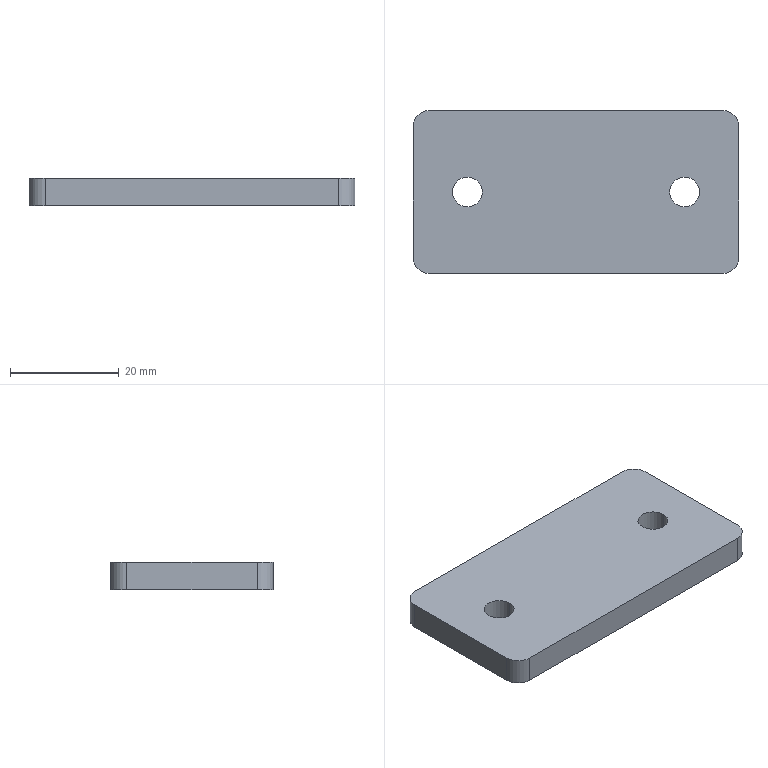Part | STEP file | Guide wheel mechanism revised.sldasm-Part-42 | 1 solid | 14 faces | box 60 x 30 x 5 mm | volume 8724 mm3 | cylinder 8 | plane 6 | commonest cylinder face diameters 5.5 x4 6 x4
STEP:
#1=CARTESIAN_POINT('',(-17.25,0.,-2.5));
#2=VERTEX_POINT('',#1);
#3=CARTESIAN_POINT('',(-22.75,0.,-2.5));
#4=VERTEX_POINT('',#3);
#5=CARTESIAN_POINT('',(-20.,0.,-2.5));
#6=DIRECTION('',(0.,0.,-1.));
#7=DIRECTION('',(-1.,0.,0.));
#8=AXIS2_PLACEMENT_3D('',#5,#6,#7);
#9=CIRCLE('',#8,2.75);
#10=EDGE_CURVE('',#2,#4,#9,.T.);
#11=ORIENTED_EDGE('',*,*,#10,.T.);
#12=CARTESIAN_POINT('',(-22.75,0.,2.5));
#13=VERTEX_POINT('',#12);
#14=CARTESIAN_POINT('',(-22.75,0.,2.5));
#15=DIRECTION('',(0.,0.,1.));
#16=VECTOR('',#15,1000.);
#17=LINE('',#14,#16);
#18=EDGE_CURVE('',#4,#13,#17,.T.);
#19=ORIENTED_EDGE('',*,*,#18,.T.);
#20=CARTESIAN_POINT('',(-17.25,0.,2.5));
#21=VERTEX_POINT('',#20);
#22=CARTESIAN_POINT('',(-20.,0.,2.5));
#23=DIRECTION('',(0.,0.,1.));
#24=DIRECTION('',(1.,0.,0.));
#25=AXIS2_PLACEMENT_3D('',#22,#23,#24);
#26=CIRCLE('',#25,2.75);
#27=EDGE_CURVE('',#13,#21,#26,.T.);
#28=ORIENTED_EDGE('',*,*,#27,.T.);
#29=CARTESIAN_POINT('',(-17.25,0.,2.5));
#30=DIRECTION('',(0.,0.,1.));
#31=VECTOR('',#30,1000.);
#32=LINE('',#29,#31);
#33=EDGE_CURVE('',#2,#21,#32,.T.);
#34=ORIENTED_EDGE('',*,*,#33,.F.);
#35=EDGE_LOOP('',(#11,#19,#28,#34));
#36=FACE_OUTER_BOUND('',#35,.T.);
#37=CARTESIAN_POINT('',(-20.,0.,2.5));
#38=DIRECTION('',(0.,0.,1.));
#39=DIRECTION('',(1.,0.,0.));
#40=AXIS2_PLACEMENT_3D('',#37,#38,#39);
#41=CYLINDRICAL_SURFACE('',#40,2.75);
#42=ADVANCED_FACE('',(#36),#41,.F.);
#43=CARTESIAN_POINT('',(22.75,0.,-2.5));
#44=VERTEX_POINT('',#43);
#45=CARTESIAN_POINT('',(17.25,0.,-2.5));
#46=VERTEX_POINT('',#45);
#47=CARTESIAN_POINT('',(20.,0.,-2.5));
#48=DIRECTION('',(0.,0.,-1.));
#49=DIRECTION('',(-1.,0.,0.));
#50=AXIS2_PLACEMENT_3D('',#47,#48,#49);
#51=CIRCLE('',#50,2.75);
#52=EDGE_CURVE('',#44,#46,#51,.T.);
#53=ORIENTED_EDGE('',*,*,#52,.T.);
#54=CARTESIAN_POINT('',(17.25,0.,2.5));
#55=VERTEX_POINT('',#54);
#56=CARTESIAN_POINT('',(17.25,0.,2.5));
#57=DIRECTION('',(0.,0.,1.));
#58=VECTOR('',#57,1000.);
#59=LINE('',#56,#58);
#60=EDGE_CURVE('',#46,#55,#59,.T.);
#61=ORIENTED_EDGE('',*,*,#60,.T.);
#62=CARTESIAN_POINT('',(22.75,0.,2.5));
#63=VERTEX_POINT('',#62);
#64=CARTESIAN_POINT('',(20.,0.,2.5));
#65=DIRECTION('',(0.,0.,1.));
#66=DIRECTION('',(1.,0.,0.));
#67=AXIS2_PLACEMENT_3D('',#64,#65,#66);
#68=CIRCLE('',#67,2.75);
#69=EDGE_CURVE('',#55,#63,#68,.T.);
#70=ORIENTED_EDGE('',*,*,#69,.T.);
#71=CARTESIAN_POINT('',(22.75,0.,2.5));
#72=DIRECTION('',(0.,0.,1.));
#73=VECTOR('',#72,1000.);
#74=LINE('',#71,#73);
#75=EDGE_CURVE('',#44,#63,#74,.T.);
#76=ORIENTED_EDGE('',*,*,#75,.F.);
#77=EDGE_LOOP('',(#53,#61,#70,#76));
#78=FACE_OUTER_BOUND('',#77,.T.);
#79=CARTESIAN_POINT('',(20.,0.,2.5));
#80=DIRECTION('',(0.,0.,1.));
#81=DIRECTION('',(1.,0.,0.));
#82=AXIS2_PLACEMENT_3D('',#79,#80,#81);
#83=CYLINDRICAL_SURFACE('',#82,2.75);
#84=ADVANCED_FACE('',(#78),#83,.F.);
#85=CARTESIAN_POINT('',(30.,-12.,2.5));
#86=VERTEX_POINT('',#85);
#87=CARTESIAN_POINT('',(30.,12.,2.5));
#88=VERTEX_POINT('',#87);
#89=CARTESIAN_POINT('',(30.,-15.,2.5));
#90=DIRECTION('',(0.,1.,0.));
#91=VECTOR('',#90,1000.);
#92=LINE('',#89,#91);
#93=EDGE_CURVE('',#86,#88,#92,.T.);
#94=ORIENTED_EDGE('',*,*,#93,.F.);
#95=CARTESIAN_POINT('',(30.,-12.,-2.5));
#96=VERTEX_POINT('',#95);
#97=CARTESIAN_POINT('',(30.,-12.,2.5));
#98=DIRECTION('',(0.,0.,-1.));
#99=VECTOR('',#98,1000.);
#100=LINE('',#97,#99);
#101=EDGE_CURVE('',#86,#96,#100,.T.);
#102=ORIENTED_EDGE('',*,*,#101,.T.);
#103=CARTESIAN_POINT('',(30.,12.,-2.5));
#104=VERTEX_POINT('',#103);
#105=CARTESIAN_POINT('',(30.,-15.,-2.5));
#106=DIRECTION('',(0.,1.,0.));
#107=VECTOR('',#106,1000.);
#108=LINE('',#105,#107);
#109=EDGE_CURVE('',#96,#104,#108,.T.);
#110=ORIENTED_EDGE('',*,*,#109,.T.);
#111=CARTESIAN_POINT('',(30.,12.,2.5));
#112=DIRECTION('',(0.,0.,1.));
#113=VECTOR('',#112,1000.);
#114=LINE('',#111,#113);
#115=EDGE_CURVE('',#104,#88,#114,.T.);
#116=ORIENTED_EDGE('',*,*,#115,.T.);
#117=EDGE_LOOP('',(#94,#102,#110,#116));
#118=FACE_OUTER_BOUND('',#117,.T.);
#119=CARTESIAN_POINT('',(30.,-15.,2.5));
#120=DIRECTION('',(-1.,0.,0.));
#121=DIRECTION('',(0.,0.,1.));
#122=AXIS2_PLACEMENT_3D('',#119,#120,#121);
#123=PLANE('',#122);
#124=ADVANCED_FACE('',(#118),#123,.F.);
#125=CARTESIAN_POINT('',(27.,15.,-2.5));
#126=VERTEX_POINT('',#125);
#127=CARTESIAN_POINT('',(-27.,15.,-2.5));
#128=VERTEX_POINT('',#127);
#129=CARTESIAN_POINT('',(-30.,15.,-2.5));
#130=DIRECTION('',(-1.,0.,0.));
#131=VECTOR('',#130,1000.);
#132=LINE('',#129,#131);
#133=EDGE_CURVE('',#126,#128,#132,.T.);
#134=ORIENTED_EDGE('',*,*,#133,.T.);
#135=CARTESIAN_POINT('',(-27.,15.,2.5));
#136=VERTEX_POINT('',#135);
#137=CARTESIAN_POINT('',(-27.,15.,2.5));
#138=DIRECTION('',(0.,0.,1.));
#139=VECTOR('',#138,1000.);
#140=LINE('',#137,#139);
#141=EDGE_CURVE('',#128,#136,#140,.T.);
#142=ORIENTED_EDGE('',*,*,#141,.T.);
#143=CARTESIAN_POINT('',(27.,15.,2.5));
#144=VERTEX_POINT('',#143);
#145=CARTESIAN_POINT('',(-30.,15.,2.5));
#146=DIRECTION('',(-1.,0.,0.));
#147=VECTOR('',#146,1000.);
#148=LINE('',#145,#147);
#149=EDGE_CURVE('',#144,#136,#148,.T.);
#150=ORIENTED_EDGE('',*,*,#149,.F.);
#151=CARTESIAN_POINT('',(27.,15.,2.5));
#152=DIRECTION('',(0.,0.,-1.));
#153=VECTOR('',#152,1000.);
#154=LINE('',#151,#153);
#155=EDGE_CURVE('',#144,#126,#154,.T.);
#156=ORIENTED_EDGE('',*,*,#155,.T.);
#157=EDGE_LOOP('',(#134,#142,#150,#156));
#158=FACE_OUTER_BOUND('',#157,.T.);
#159=CARTESIAN_POINT('',(-30.,15.,2.5));
#160=DIRECTION('',(0.,-1.,0.));
#161=DIRECTION('',(0.,0.,-1.));
#162=AXIS2_PLACEMENT_3D('',#159,#160,#161);
#163=PLANE('',#162);
#164=ADVANCED_FACE('',(#158),#163,.F.);
#165=CARTESIAN_POINT('',(-30.,12.,-2.5));
#166=VERTEX_POINT('',#165);
#167=CARTESIAN_POINT('',(-30.,-12.,-2.5));
#168=VERTEX_POINT('',#167);
#169=CARTESIAN_POINT('',(-30.,-15.,-2.5));
#170=DIRECTION('',(0.,-1.,0.));
#171=VECTOR('',#170,1000.);
#172=LINE('',#169,#171);
#173=EDGE_CURVE('',#166,#168,#172,.T.);
#174=ORIENTED_EDGE('',*,*,#173,.T.);
#175=CARTESIAN_POINT('',(-30.,-12.,2.5));
#176=VERTEX_POINT('',#175);
#177=CARTESIAN_POINT('',(-30.,-12.,2.5));
#178=DIRECTION('',(0.,0.,1.));
#179=VECTOR('',#178,1000.);
#180=LINE('',#177,#179);
#181=EDGE_CURVE('',#168,#176,#180,.T.);
#182=ORIENTED_EDGE('',*,*,#181,.T.);
#183=CARTESIAN_POINT('',(-30.,12.,2.5));
#184=VERTEX_POINT('',#183);
#185=CARTESIAN_POINT('',(-30.,-15.,2.5));
#186=DIRECTION('',(0.,-1.,0.));
#187=VECTOR('',#186,1000.);
#188=LINE('',#185,#187);
#189=EDGE_CURVE('',#184,#176,#188,.T.);
#190=ORIENTED_EDGE('',*,*,#189,.F.);
#191=CARTESIAN_POINT('',(-30.,12.,2.5));
#192=DIRECTION('',(0.,0.,-1.));
#193=VECTOR('',#192,1000.);
#194=LINE('',#191,#193);
#195=EDGE_CURVE('',#184,#166,#194,.T.);
#196=ORIENTED_EDGE('',*,*,#195,.T.);
#197=EDGE_LOOP('',(#174,#182,#190,#196));
#198=FACE_OUTER_BOUND('',#197,.T.);
#199=CARTESIAN_POINT('',(-30.,-15.,2.5));
#200=DIRECTION('',(1.,0.,0.));
#201=DIRECTION('',(0.,0.,-1.));
#202=AXIS2_PLACEMENT_3D('',#199,#200,#201);
#203=PLANE('',#202);
#204=ADVANCED_FACE('',(#198),#203,.F.);
#205=CARTESIAN_POINT('',(-27.,-15.,2.5));
#206=VERTEX_POINT('',#205);
#207=CARTESIAN_POINT('',(27.,-15.,2.5));
#208=VERTEX_POINT('',#207);
#209=CARTESIAN_POINT('',(-30.,-15.,2.5));
#210=DIRECTION('',(1.,0.,0.));
#211=VECTOR('',#210,1000.);
#212=LINE('',#209,#211);
#213=EDGE_CURVE('',#206,#208,#212,.T.);
#214=ORIENTED_EDGE('',*,*,#213,.F.);
#215=CARTESIAN_POINT('',(-27.,-15.,-2.5));
#216=VERTEX_POINT('',#215);
#217=CARTESIAN_POINT('',(-27.,-15.,2.5));
#218=DIRECTION('',(0.,0.,-1.));
#219=VECTOR('',#218,1000.);
#220=LINE('',#217,#219);
#221=EDGE_CURVE('',#206,#216,#220,.T.);
#222=ORIENTED_EDGE('',*,*,#221,.T.);
#223=CARTESIAN_POINT('',(27.,-15.,-2.5));
#224=VERTEX_POINT('',#223);
#225=CARTESIAN_POINT('',(-30.,-15.,-2.5));
#226=DIRECTION('',(1.,0.,0.));
#227=VECTOR('',#226,1000.);
#228=LINE('',#225,#227);
#229=EDGE_CURVE('',#216,#224,#228,.T.);
#230=ORIENTED_EDGE('',*,*,#229,.T.);
#231=CARTESIAN_POINT('',(27.,-15.,2.5));
#232=DIRECTION('',(0.,0.,1.));
#233=VECTOR('',#232,1000.);
#234=LINE('',#231,#233);
#235=EDGE_CURVE('',#224,#208,#234,.T.);
#236=ORIENTED_EDGE('',*,*,#235,.T.);
#237=EDGE_LOOP('',(#214,#222,#230,#236));
#238=FACE_OUTER_BOUND('',#237,.T.);
#239=CARTESIAN_POINT('',(-30.,-15.,2.5));
#240=DIRECTION('',(0.,1.,0.));
#241=DIRECTION('',(0.,0.,1.));
#242=AXIS2_PLACEMENT_3D('',#239,#240,#241);
#243=PLANE('',#242);
#244=ADVANCED_FACE('',(#238),#243,.F.);
#245=CARTESIAN_POINT('',(-20.,0.,2.5));
#246=DIRECTION('',(0.,0.,1.));
#247=DIRECTION('',(1.,0.,0.));
#248=AXIS2_PLACEMENT_3D('',#245,#246,#247);
#249=CIRCLE('',#248,2.75);
#250=EDGE_CURVE('',#21,#13,#249,.T.);
#251=ORIENTED_EDGE('',*,*,#250,.F.);
#252=ORIENTED_EDGE('',*,*,#27,.F.);
#253=EDGE_LOOP('',(#251,#252));
#254=FACE_BOUND('',#253,.T.);
#255=CARTESIAN_POINT('',(20.,0.,2.5));
#256=DIRECTION('',(0.,0.,1.));
#257=DIRECTION('',(1.,0.,0.));
#258=AXIS2_PLACEMENT_3D('',#255,#256,#257);
#259=CIRCLE('',#258,2.75);
#260=EDGE_CURVE('',#63,#55,#259,.T.);
#261=ORIENTED_EDGE('',*,*,#260,.F.);
#262=ORIENTED_EDGE('',*,*,#69,.F.);
#263=EDGE_LOOP('',(#261,#262));
#264=FACE_BOUND('',#263,.T.);
#265=ORIENTED_EDGE('',*,*,#189,.T.);
#266=CARTESIAN_POINT('',(-27.,-12.,2.5));
#267=DIRECTION('',(0.,0.,1.));
#268=DIRECTION('',(-1.,0.,0.));
#269=AXIS2_PLACEMENT_3D('',#266,#267,#268);
#270=CIRCLE('',#269,3.);
#271=EDGE_CURVE('',#176,#206,#270,.T.);
#272=ORIENTED_EDGE('',*,*,#271,.T.);
#273=ORIENTED_EDGE('',*,*,#213,.T.);
#274=CARTESIAN_POINT('',(27.,-12.,2.5));
#275=DIRECTION('',(0.,0.,1.));
#276=DIRECTION('',(-1.,0.,0.));
#277=AXIS2_PLACEMENT_3D('',#274,#275,#276);
#278=CIRCLE('',#277,3.);
#279=EDGE_CURVE('',#208,#86,#278,.T.);
#280=ORIENTED_EDGE('',*,*,#279,.T.);
#281=ORIENTED_EDGE('',*,*,#93,.T.);
#282=CARTESIAN_POINT('',(27.,12.,2.5));
#283=DIRECTION('',(0.,0.,1.));
#284=DIRECTION('',(-1.,0.,0.));
#285=AXIS2_PLACEMENT_3D('',#282,#283,#284);
#286=CIRCLE('',#285,3.);
#287=EDGE_CURVE('',#88,#144,#286,.T.);
#288=ORIENTED_EDGE('',*,*,#287,.T.);
#289=ORIENTED_EDGE('',*,*,#149,.T.);
#290=CARTESIAN_POINT('',(-27.,12.,2.5));
#291=DIRECTION('',(0.,0.,1.));
#292=DIRECTION('',(-1.,0.,0.));
#293=AXIS2_PLACEMENT_3D('',#290,#291,#292);
#294=CIRCLE('',#293,3.);
#295=EDGE_CURVE('',#136,#184,#294,.T.);
#296=ORIENTED_EDGE('',*,*,#295,.T.);
#297=EDGE_LOOP('',(#265,#272,#273,#280,#281,#288,#289,#296));
#298=FACE_OUTER_BOUND('',#297,.T.);
#299=CARTESIAN_POINT('',(0.,0.,2.5));
#300=DIRECTION('',(0.,0.,-1.));
#301=DIRECTION('',(-1.,0.,0.));
#302=AXIS2_PLACEMENT_3D('',#299,#300,#301);
#303=PLANE('',#302);
#304=ADVANCED_FACE('',(#254,#264,#298),#303,.F.);
#305=ORIENTED_EDGE('',*,*,#10,.F.);
#306=CARTESIAN_POINT('',(-20.,0.,-2.5));
#307=DIRECTION('',(0.,0.,-1.));
#308=DIRECTION('',(-1.,0.,0.));
#309=AXIS2_PLACEMENT_3D('',#306,#307,#308);
#310=CIRCLE('',#309,2.75);
#311=EDGE_CURVE('',#4,#2,#310,.T.);
#312=ORIENTED_EDGE('',*,*,#311,.F.);
#313=EDGE_LOOP('',(#305,#312));
#314=FACE_BOUND('',#313,.T.);
#315=ORIENTED_EDGE('',*,*,#52,.F.);
#316=CARTESIAN_POINT('',(20.,0.,-2.5));
#317=DIRECTION('',(0.,0.,-1.));
#318=DIRECTION('',(-1.,0.,0.));
#319=AXIS2_PLACEMENT_3D('',#316,#317,#318);
#320=CIRCLE('',#319,2.75);
#321=EDGE_CURVE('',#46,#44,#320,.T.);
#322=ORIENTED_EDGE('',*,*,#321,.F.);
#323=EDGE_LOOP('',(#315,#322));
#324=FACE_BOUND('',#323,.T.);
#325=ORIENTED_EDGE('',*,*,#229,.F.);
#326=CARTESIAN_POINT('',(-27.,-12.,-2.5));
#327=DIRECTION('',(0.,0.,-1.));
#328=DIRECTION('',(-1.,0.,0.));
#329=AXIS2_PLACEMENT_3D('',#326,#327,#328);
#330=CIRCLE('',#329,3.);
#331=EDGE_CURVE('',#216,#168,#330,.T.);
#332=ORIENTED_EDGE('',*,*,#331,.T.);
#333=ORIENTED_EDGE('',*,*,#173,.F.);
#334=CARTESIAN_POINT('',(-27.,12.,-2.5));
#335=DIRECTION('',(0.,0.,-1.));
#336=DIRECTION('',(-1.,0.,0.));
#337=AXIS2_PLACEMENT_3D('',#334,#335,#336);
#338=CIRCLE('',#337,3.);
#339=EDGE_CURVE('',#166,#128,#338,.T.);
#340=ORIENTED_EDGE('',*,*,#339,.T.);
#341=ORIENTED_EDGE('',*,*,#133,.F.);
#342=CARTESIAN_POINT('',(27.,12.,-2.5));
#343=DIRECTION('',(0.,0.,-1.));
#344=DIRECTION('',(-1.,0.,0.));
#345=AXIS2_PLACEMENT_3D('',#342,#343,#344);
#346=CIRCLE('',#345,3.);
#347=EDGE_CURVE('',#126,#104,#346,.T.);
#348=ORIENTED_EDGE('',*,*,#347,.T.);
#349=ORIENTED_EDGE('',*,*,#109,.F.);
#350=CARTESIAN_POINT('',(27.,-12.,-2.5));
#351=DIRECTION('',(0.,0.,-1.));
#352=DIRECTION('',(-1.,0.,0.));
#353=AXIS2_PLACEMENT_3D('',#350,#351,#352);
#354=CIRCLE('',#353,3.);
#355=EDGE_CURVE('',#96,#224,#354,.T.);
#356=ORIENTED_EDGE('',*,*,#355,.T.);
#357=EDGE_LOOP('',(#325,#332,#333,#340,#341,#348,#349,#356));
#358=FACE_OUTER_BOUND('',#357,.T.);
#359=CARTESIAN_POINT('',(0.,0.,-2.5));
#360=DIRECTION('',(0.,0.,-1.));
#361=DIRECTION('',(-1.,0.,0.));
#362=AXIS2_PLACEMENT_3D('',#359,#360,#361);
#363=PLANE('',#362);
#364=ADVANCED_FACE('',(#314,#324,#358),#363,.T.);
#365=ORIENTED_EDGE('',*,*,#60,.F.);
#366=ORIENTED_EDGE('',*,*,#321,.T.);
#367=ORIENTED_EDGE('',*,*,#75,.T.);
#368=ORIENTED_EDGE('',*,*,#260,.T.);
#369=EDGE_LOOP('',(#365,#366,#367,#368));
#370=FACE_OUTER_BOUND('',#369,.T.);
#371=CARTESIAN_POINT('',(20.,0.,2.5));
#372=DIRECTION('',(0.,0.,1.));
#373=DIRECTION('',(1.,0.,0.));
#374=AXIS2_PLACEMENT_3D('',#371,#372,#373);
#375=CYLINDRICAL_SURFACE('',#374,2.75);
#376=ADVANCED_FACE('',(#370),#375,.F.);
#377=ORIENTED_EDGE('',*,*,#18,.F.);
#378=ORIENTED_EDGE('',*,*,#311,.T.);
#379=ORIENTED_EDGE('',*,*,#33,.T.);
#380=ORIENTED_EDGE('',*,*,#250,.T.);
#381=EDGE_LOOP('',(#377,#378,#379,#380));
#382=FACE_OUTER_BOUND('',#381,.T.);
#383=CARTESIAN_POINT('',(-20.,0.,2.5));
#384=DIRECTION('',(0.,0.,1.));
#385=DIRECTION('',(1.,0.,0.));
#386=AXIS2_PLACEMENT_3D('',#383,#384,#385);
#387=CYLINDRICAL_SURFACE('',#386,2.75);
#388=ADVANCED_FACE('',(#382),#387,.F.);
#389=ORIENTED_EDGE('',*,*,#271,.F.);
#390=ORIENTED_EDGE('',*,*,#181,.F.);
#391=ORIENTED_EDGE('',*,*,#331,.F.);
#392=ORIENTED_EDGE('',*,*,#221,.F.);
#393=EDGE_LOOP('',(#389,#390,#391,#392));
#394=FACE_OUTER_BOUND('',#393,.T.);
#395=CARTESIAN_POINT('',(-27.,-12.,2.5));
#396=DIRECTION('',(0.,0.,-1.));
#397=DIRECTION('',(-1.,0.,0.));
#398=AXIS2_PLACEMENT_3D('',#395,#396,#397);
#399=CYLINDRICAL_SURFACE('',#398,3.);
#400=ADVANCED_FACE('',(#394),#399,.T.);
#401=ORIENTED_EDGE('',*,*,#279,.F.);
#402=ORIENTED_EDGE('',*,*,#235,.F.);
#403=ORIENTED_EDGE('',*,*,#355,.F.);
#404=ORIENTED_EDGE('',*,*,#101,.F.);
#405=EDGE_LOOP('',(#401,#402,#403,#404));
#406=FACE_OUTER_BOUND('',#405,.T.);
#407=CARTESIAN_POINT('',(27.,-12.,2.5));
#408=DIRECTION('',(0.,0.,-1.));
#409=DIRECTION('',(-1.,0.,0.));
#410=AXIS2_PLACEMENT_3D('',#407,#408,#409);
#411=CYLINDRICAL_SURFACE('',#410,3.);
#412=ADVANCED_FACE('',(#406),#411,.T.);
#413=ORIENTED_EDGE('',*,*,#295,.F.);
#414=ORIENTED_EDGE('',*,*,#141,.F.);
#415=ORIENTED_EDGE('',*,*,#339,.F.);
#416=ORIENTED_EDGE('',*,*,#195,.F.);
#417=EDGE_LOOP('',(#413,#414,#415,#416));
#418=FACE_OUTER_BOUND('',#417,.T.);
#419=CARTESIAN_POINT('',(-27.,12.,2.5));
#420=DIRECTION('',(0.,0.,-1.));
#421=DIRECTION('',(-1.,0.,0.));
#422=AXIS2_PLACEMENT_3D('',#419,#420,#421);
#423=CYLINDRICAL_SURFACE('',#422,3.);
#424=ADVANCED_FACE('',(#418),#423,.T.);
#425=ORIENTED_EDGE('',*,*,#287,.F.);
#426=ORIENTED_EDGE('',*,*,#115,.F.);
#427=ORIENTED_EDGE('',*,*,#347,.F.);
#428=ORIENTED_EDGE('',*,*,#155,.F.);
#429=EDGE_LOOP('',(#425,#426,#427,#428));
#430=FACE_OUTER_BOUND('',#429,.T.);
#431=CARTESIAN_POINT('',(27.,12.,2.5));
#432=DIRECTION('',(0.,0.,-1.));
#433=DIRECTION('',(-1.,0.,0.));
#434=AXIS2_PLACEMENT_3D('',#431,#432,#433);
#435=CYLINDRICAL_SURFACE('',#434,3.);
#436=ADVANCED_FACE('',(#430),#435,.T.);
#437=CLOSED_SHELL('',(#42,#84,#124,#164,#204,#244,#304,#364,#376,#388,#400,#412,#424,#436));
#438=MANIFOLD_SOLID_BREP('',#437);
#439=CARTESIAN_POINT('',(0.,0.,0.));
#440=DIRECTION('',(0.,0.,1.));
#441=DIRECTION('',(1.,0.,0.));
#442=AXIS2_PLACEMENT_3D('',#439,#440,#441);
#443=(LENGTH_UNIT()NAMED_UNIT(*)SI_UNIT(.MILLI.,.METRE.));
#444=UNCERTAINTY_MEASURE_WITH_UNIT(LENGTH_MEASURE(0.00001),#443,'','');
#445=(NAMED_UNIT(*)PLANE_ANGLE_UNIT()SI_UNIT($,.RADIAN.));
#446=(NAMED_UNIT(*)SI_UNIT($,.STERADIAN.)SOLID_ANGLE_UNIT());
#447=(GEOMETRIC_REPRESENTATION_CONTEXT(3)GLOBAL_UNCERTAINTY_ASSIGNED_CONTEXT((#444))GLOBAL_UNIT_ASSIGNED_CONTEXT((#443,#445,#446))REPRESENTATION_CONTEXT('',''));
#448=ADVANCED_BREP_SHAPE_REPRESENTATION('',(#438,#442),#447);